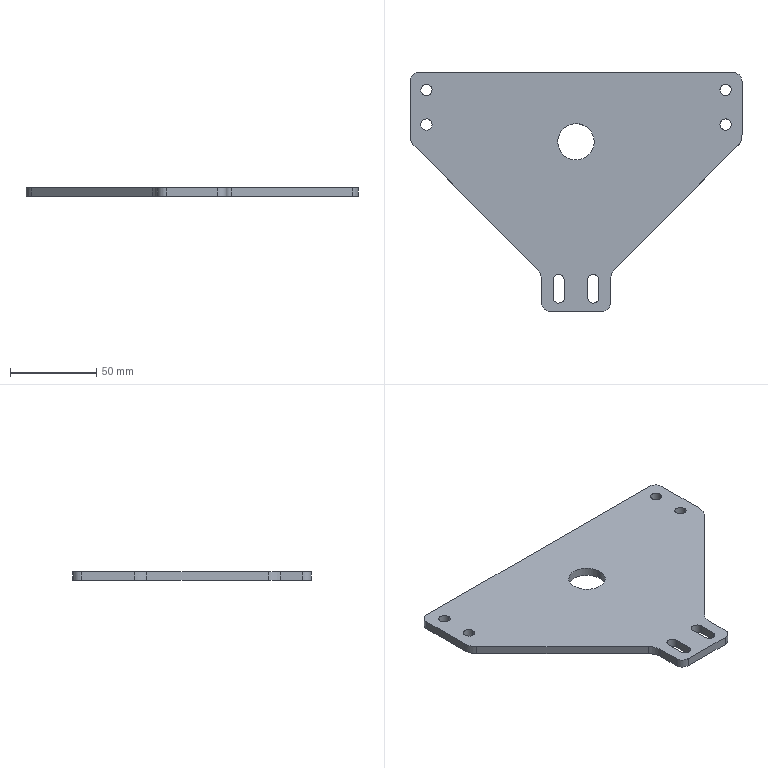Part | STEP file | 101000007795 | 1 solid | 36 faces | box 192 x 138 x 5 mm | volume 83395 mm3 | cylinder 22 | plane 14 | commonest cylinder face diameters 6.5 x12 10 x4 20 x4 21 x2